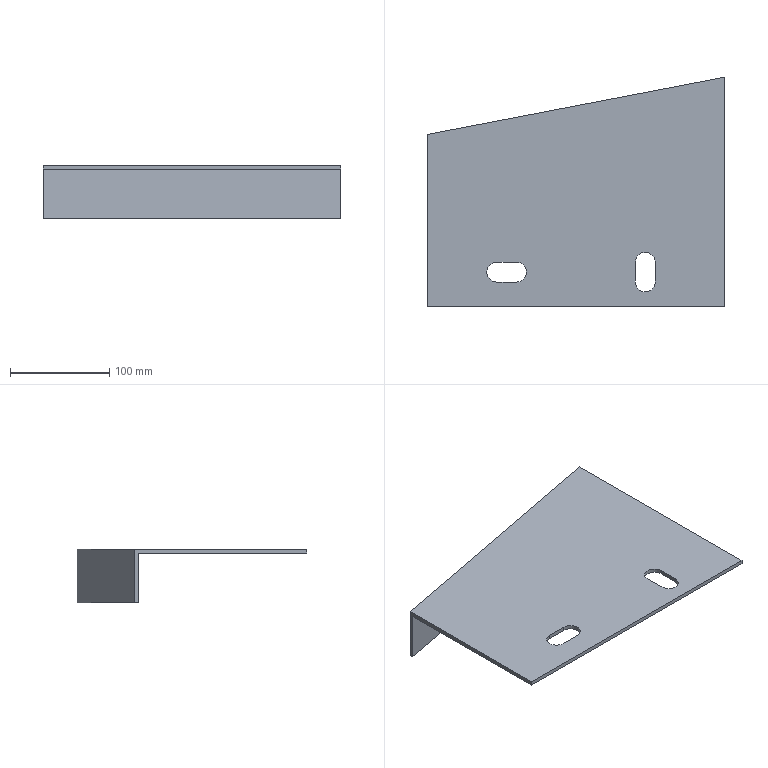Part | SolidWorks | features MirrorStock 1 | 1 solid | 17 faces | box 300 x 231.743 x 54 mm | volume 298834 mm3 | plane 12 | cylinder 5 | commonest cylinder face diameters 20 x5
STEP:
#1=CARTESIAN_POINT('',(60.,35.,-4.));
#2=VERTEX_POINT('',#1);
#3=CARTESIAN_POINT('',(70.,25.,-4.));
#4=VERTEX_POINT('',#3);
#5=CARTESIAN_POINT('',(70.,35.,-4.));
#6=DIRECTION('',(0.,0.,1.));
#7=DIRECTION('',(1.,0.,0.));
#8=AXIS2_PLACEMENT_3D('',#5,#6,#7);
#9=CIRCLE('',#8,10.);
#10=EDGE_CURVE('',#2,#4,#9,.T.);
#11=ORIENTED_EDGE('',*,*,#10,.F.);
#12=CARTESIAN_POINT('',(60.,35.,0.));
#13=VERTEX_POINT('',#12);
#14=CARTESIAN_POINT('',(60.,35.,-4.));
#15=DIRECTION('',(0.,0.,1.));
#16=VECTOR('',#15,1000.);
#17=LINE('',#14,#16);
#18=EDGE_CURVE('',#2,#13,#17,.T.);
#19=ORIENTED_EDGE('',*,*,#18,.T.);
#20=CARTESIAN_POINT('',(70.,25.,0.));
#21=VERTEX_POINT('',#20);
#22=CARTESIAN_POINT('',(70.,35.,0.));
#23=DIRECTION('',(0.,0.,1.));
#24=DIRECTION('',(1.,0.,0.));
#25=AXIS2_PLACEMENT_3D('',#22,#23,#24);
#26=CIRCLE('',#25,10.);
#27=EDGE_CURVE('',#13,#21,#26,.T.);
#28=ORIENTED_EDGE('',*,*,#27,.T.);
#29=CARTESIAN_POINT('',(70.,25.,-4.));
#30=DIRECTION('',(0.,0.,1.));
#31=VECTOR('',#30,1000.);
#32=LINE('',#29,#31);
#33=EDGE_CURVE('',#4,#21,#32,.T.);
#34=ORIENTED_EDGE('',*,*,#33,.F.);
#35=EDGE_LOOP('',(#11,#19,#28,#34));
#36=FACE_OUTER_BOUND('',#35,.T.);
#37=CARTESIAN_POINT('',(70.,35.,-4.));
#38=DIRECTION('',(0.,0.,1.));
#39=DIRECTION('',(-1.,0.,0.));
#40=AXIS2_PLACEMENT_3D('',#37,#38,#39);
#41=CYLINDRICAL_SURFACE('',#40,10.);
#42=ADVANCED_FACE('',(#36),#41,.F.);
#43=CARTESIAN_POINT('',(0.,169.927,-4.));
#44=VERTEX_POINT('',#43);
#45=CARTESIAN_POINT('',(300.,227.669,-4.));
#46=VERTEX_POINT('',#45);
#47=CARTESIAN_POINT('',(21.163,174.,-4.));
#48=DIRECTION('',(0.982,0.189,0.));
#49=VECTOR('',#48,1000.);
#50=LINE('',#47,#49);
#51=EDGE_CURVE('',#44,#46,#50,.T.);
#52=ORIENTED_EDGE('',*,*,#51,.T.);
#53=CARTESIAN_POINT('',(300.,0.,-4.));
#54=VERTEX_POINT('',#53);
#55=CARTESIAN_POINT('',(300.,231.743,-4.));
#56=DIRECTION('',(0.,1.,0.));
#57=VECTOR('',#56,1000.);
#58=LINE('',#55,#57);
#59=EDGE_CURVE('',#54,#46,#58,.T.);
#60=ORIENTED_EDGE('',*,*,#59,.F.);
#61=CARTESIAN_POINT('',(0.,0.,-4.));
#62=VERTEX_POINT('',#61);
#63=CARTESIAN_POINT('',(300.,0.,-4.));
#64=DIRECTION('',(1.,0.,0.));
#65=VECTOR('',#64,1000.);
#66=LINE('',#63,#65);
#67=EDGE_CURVE('',#62,#54,#66,.T.);
#68=ORIENTED_EDGE('',*,*,#67,.F.);
#69=CARTESIAN_POINT('',(0.,0.,-4.));
#70=DIRECTION('',(0.,-1.,0.));
#71=VECTOR('',#70,1000.);
#72=LINE('',#69,#71);
#73=EDGE_CURVE('',#44,#62,#72,.T.);
#74=ORIENTED_EDGE('',*,*,#73,.F.);
#75=EDGE_LOOP('',(#52,#60,#68,#74));
#76=FACE_OUTER_BOUND('',#75,.T.);
#77=CARTESIAN_POINT('',(90.,25.,-4.));
#78=VERTEX_POINT('',#77);
#79=CARTESIAN_POINT('',(90.,25.,-4.));
#80=DIRECTION('',(1.,0.,0.));
#81=VECTOR('',#80,1000.);
#82=LINE('',#79,#81);
#83=EDGE_CURVE('',#4,#78,#82,.T.);
#84=ORIENTED_EDGE('',*,*,#83,.T.);
#85=CARTESIAN_POINT('',(90.,45.,-4.));
#86=VERTEX_POINT('',#85);
#87=CARTESIAN_POINT('',(90.,35.,-4.));
#88=DIRECTION('',(0.,0.,1.));
#89=DIRECTION('',(1.,0.,0.));
#90=AXIS2_PLACEMENT_3D('',#87,#88,#89);
#91=CIRCLE('',#90,10.);
#92=EDGE_CURVE('',#78,#86,#91,.T.);
#93=ORIENTED_EDGE('',*,*,#92,.T.);
#94=CARTESIAN_POINT('',(70.,45.,-4.));
#95=VERTEX_POINT('',#94);
#96=CARTESIAN_POINT('',(70.,45.,-4.));
#97=DIRECTION('',(-1.,0.,0.));
#98=VECTOR('',#97,1000.);
#99=LINE('',#96,#98);
#100=EDGE_CURVE('',#86,#95,#99,.T.);
#101=ORIENTED_EDGE('',*,*,#100,.T.);
#102=CARTESIAN_POINT('',(70.,35.,-4.));
#103=DIRECTION('',(0.,0.,1.));
#104=DIRECTION('',(1.,0.,0.));
#105=AXIS2_PLACEMENT_3D('',#102,#103,#104);
#106=CIRCLE('',#105,10.);
#107=EDGE_CURVE('',#95,#2,#106,.T.);
#108=ORIENTED_EDGE('',*,*,#107,.T.);
#109=ORIENTED_EDGE('',*,*,#10,.T.);
#110=EDGE_LOOP('',(#84,#93,#101,#108,#109));
#111=FACE_BOUND('',#110,.T.);
#112=CARTESIAN_POINT('',(210.,45.,-4.));
#113=VERTEX_POINT('',#112);
#114=CARTESIAN_POINT('',(210.,25.,-4.));
#115=VERTEX_POINT('',#114);
#116=CARTESIAN_POINT('',(210.,25.,-4.));
#117=DIRECTION('',(0.,-1.,0.));
#118=VECTOR('',#117,1000.);
#119=LINE('',#116,#118);
#120=EDGE_CURVE('',#113,#115,#119,.T.);
#121=ORIENTED_EDGE('',*,*,#120,.T.);
#122=CARTESIAN_POINT('',(230.,25.,-4.));
#123=VERTEX_POINT('',#122);
#124=CARTESIAN_POINT('',(220.,25.,-4.));
#125=DIRECTION('',(0.,0.,1.));
#126=DIRECTION('',(1.,0.,0.));
#127=AXIS2_PLACEMENT_3D('',#124,#125,#126);
#128=CIRCLE('',#127,10.);
#129=EDGE_CURVE('',#115,#123,#128,.T.);
#130=ORIENTED_EDGE('',*,*,#129,.T.);
#131=CARTESIAN_POINT('',(230.,45.,-4.));
#132=VERTEX_POINT('',#131);
#133=CARTESIAN_POINT('',(230.,45.,-4.));
#134=DIRECTION('',(0.,1.,0.));
#135=VECTOR('',#134,1000.);
#136=LINE('',#133,#135);
#137=EDGE_CURVE('',#123,#132,#136,.T.);
#138=ORIENTED_EDGE('',*,*,#137,.T.);
#139=CARTESIAN_POINT('',(220.,45.,-4.));
#140=DIRECTION('',(0.,0.,1.));
#141=DIRECTION('',(1.,0.,0.));
#142=AXIS2_PLACEMENT_3D('',#139,#140,#141);
#143=CIRCLE('',#142,10.);
#144=EDGE_CURVE('',#132,#113,#143,.T.);
#145=ORIENTED_EDGE('',*,*,#144,.T.);
#146=EDGE_LOOP('',(#121,#130,#138,#145));
#147=FACE_BOUND('',#146,.T.);
#148=CARTESIAN_POINT('',(0.,0.,-4.));
#149=DIRECTION('',(0.,0.,-1.));
#150=DIRECTION('',(1.,0.,0.));
#151=AXIS2_PLACEMENT_3D('',#148,#149,#150);
#152=PLANE('',#151);
#153=ADVANCED_FACE('',(#76,#111,#147),#152,.T.);
#154=CARTESIAN_POINT('',(70.,45.,0.));
#155=VERTEX_POINT('',#154);
#156=CARTESIAN_POINT('',(70.,35.,0.));
#157=DIRECTION('',(0.,0.,1.));
#158=DIRECTION('',(1.,0.,0.));
#159=AXIS2_PLACEMENT_3D('',#156,#157,#158);
#160=CIRCLE('',#159,10.);
#161=EDGE_CURVE('',#155,#13,#160,.T.);
#162=ORIENTED_EDGE('',*,*,#161,.F.);
#163=CARTESIAN_POINT('',(90.,45.,0.));
#164=VERTEX_POINT('',#163);
#165=CARTESIAN_POINT('',(70.,45.,0.));
#166=DIRECTION('',(-1.,0.,0.));
#167=VECTOR('',#166,1000.);
#168=LINE('',#165,#167);
#169=EDGE_CURVE('',#164,#155,#168,.T.);
#170=ORIENTED_EDGE('',*,*,#169,.F.);
#171=CARTESIAN_POINT('',(90.,25.,0.));
#172=VERTEX_POINT('',#171);
#173=CARTESIAN_POINT('',(90.,35.,0.));
#174=DIRECTION('',(0.,0.,1.));
#175=DIRECTION('',(1.,0.,0.));
#176=AXIS2_PLACEMENT_3D('',#173,#174,#175);
#177=CIRCLE('',#176,10.);
#178=EDGE_CURVE('',#172,#164,#177,.T.);
#179=ORIENTED_EDGE('',*,*,#178,.F.);
#180=CARTESIAN_POINT('',(90.,25.,0.));
#181=DIRECTION('',(1.,0.,0.));
#182=VECTOR('',#181,1000.);
#183=LINE('',#180,#182);
#184=EDGE_CURVE('',#21,#172,#183,.T.);
#185=ORIENTED_EDGE('',*,*,#184,.F.);
#186=ORIENTED_EDGE('',*,*,#27,.F.);
#187=EDGE_LOOP('',(#162,#170,#179,#185,#186));
#188=FACE_BOUND('',#187,.T.);
#189=CARTESIAN_POINT('',(0.,174.,0.));
#190=VERTEX_POINT('',#189);
#191=CARTESIAN_POINT('',(0.,0.,0.));
#192=VERTEX_POINT('',#191);
#193=CARTESIAN_POINT('',(0.,0.,0.));
#194=DIRECTION('',(0.,-1.,0.));
#195=VECTOR('',#194,1000.);
#196=LINE('',#193,#195);
#197=EDGE_CURVE('',#190,#192,#196,.T.);
#198=ORIENTED_EDGE('',*,*,#197,.T.);
#199=CARTESIAN_POINT('',(300.,0.,0.));
#200=VERTEX_POINT('',#199);
#201=CARTESIAN_POINT('',(300.,0.,0.));
#202=DIRECTION('',(1.,0.,0.));
#203=VECTOR('',#202,1000.);
#204=LINE('',#201,#203);
#205=EDGE_CURVE('',#192,#200,#204,.T.);
#206=ORIENTED_EDGE('',*,*,#205,.T.);
#207=CARTESIAN_POINT('',(300.,231.743,0.));
#208=VERTEX_POINT('',#207);
#209=CARTESIAN_POINT('',(300.,231.743,0.));
#210=DIRECTION('',(0.,1.,0.));
#211=VECTOR('',#210,1000.);
#212=LINE('',#209,#211);
#213=EDGE_CURVE('',#200,#208,#212,.T.);
#214=ORIENTED_EDGE('',*,*,#213,.T.);
#215=CARTESIAN_POINT('',(0.,174.,0.));
#216=DIRECTION('',(-0.982,-0.189,0.));
#217=VECTOR('',#216,1000.);
#218=LINE('',#215,#217);
#219=EDGE_CURVE('',#208,#190,#218,.T.);
#220=ORIENTED_EDGE('',*,*,#219,.T.);
#221=EDGE_LOOP('',(#198,#206,#214,#220));
#222=FACE_OUTER_BOUND('',#221,.T.);
#223=CARTESIAN_POINT('',(230.,45.,0.));
#224=VERTEX_POINT('',#223);
#225=CARTESIAN_POINT('',(210.,45.,0.));
#226=VERTEX_POINT('',#225);
#227=CARTESIAN_POINT('',(220.,45.,0.));
#228=DIRECTION('',(0.,0.,1.));
#229=DIRECTION('',(1.,0.,0.));
#230=AXIS2_PLACEMENT_3D('',#227,#228,#229);
#231=CIRCLE('',#230,10.);
#232=EDGE_CURVE('',#224,#226,#231,.T.);
#233=ORIENTED_EDGE('',*,*,#232,.F.);
#234=CARTESIAN_POINT('',(230.,25.,0.));
#235=VERTEX_POINT('',#234);
#236=CARTESIAN_POINT('',(230.,45.,0.));
#237=DIRECTION('',(0.,1.,0.));
#238=VECTOR('',#237,1000.);
#239=LINE('',#236,#238);
#240=EDGE_CURVE('',#235,#224,#239,.T.);
#241=ORIENTED_EDGE('',*,*,#240,.F.);
#242=CARTESIAN_POINT('',(210.,25.,0.));
#243=VERTEX_POINT('',#242);
#244=CARTESIAN_POINT('',(220.,25.,0.));
#245=DIRECTION('',(0.,0.,1.));
#246=DIRECTION('',(1.,0.,0.));
#247=AXIS2_PLACEMENT_3D('',#244,#245,#246);
#248=CIRCLE('',#247,10.);
#249=EDGE_CURVE('',#243,#235,#248,.T.);
#250=ORIENTED_EDGE('',*,*,#249,.F.);
#251=CARTESIAN_POINT('',(210.,25.,0.));
#252=DIRECTION('',(0.,-1.,0.));
#253=VECTOR('',#252,1000.);
#254=LINE('',#251,#253);
#255=EDGE_CURVE('',#226,#243,#254,.T.);
#256=ORIENTED_EDGE('',*,*,#255,.F.);
#257=EDGE_LOOP('',(#233,#241,#250,#256));
#258=FACE_BOUND('',#257,.T.);
#259=CARTESIAN_POINT('',(0.,0.,0.));
#260=DIRECTION('',(0.,0.,-1.));
#261=DIRECTION('',(1.,0.,0.));
#262=AXIS2_PLACEMENT_3D('',#259,#260,#261);
#263=PLANE('',#262);
#264=ADVANCED_FACE('',(#188,#222,#258),#263,.F.);
#265=ORIENTED_EDGE('',*,*,#197,.F.);
#266=CARTESIAN_POINT('',(0.,174.,-54.));
#267=VERTEX_POINT('',#266);
#268=CARTESIAN_POINT('',(0.,174.,-4.));
#269=DIRECTION('',(0.,0.,1.));
#270=VECTOR('',#269,1000.);
#271=LINE('',#268,#270);
#272=EDGE_CURVE('',#267,#190,#271,.T.);
#273=ORIENTED_EDGE('',*,*,#272,.F.);
#274=CARTESIAN_POINT('',(0.,169.927,-54.));
#275=VERTEX_POINT('',#274);
#276=CARTESIAN_POINT('',(0.,174.,-54.));
#277=DIRECTION('',(0.,-1.,0.));
#278=VECTOR('',#277,1000.);
#279=LINE('',#276,#278);
#280=EDGE_CURVE('',#267,#275,#279,.T.);
#281=ORIENTED_EDGE('',*,*,#280,.T.);
#282=CARTESIAN_POINT('',(0.,169.927,-54.));
#283=DIRECTION('',(0.,0.,1.));
#284=VECTOR('',#283,1000.);
#285=LINE('',#282,#284);
#286=EDGE_CURVE('',#275,#44,#285,.T.);
#287=ORIENTED_EDGE('',*,*,#286,.T.);
#288=ORIENTED_EDGE('',*,*,#73,.T.);
#289=CARTESIAN_POINT('',(0.,0.,-4.));
#290=DIRECTION('',(0.,0.,1.));
#291=VECTOR('',#290,1000.);
#292=LINE('',#289,#291);
#293=EDGE_CURVE('',#62,#192,#292,.T.);
#294=ORIENTED_EDGE('',*,*,#293,.T.);
#295=EDGE_LOOP('',(#265,#273,#281,#287,#288,#294));
#296=FACE_OUTER_BOUND('',#295,.T.);
#297=CARTESIAN_POINT('',(0.,0.,-4.));
#298=DIRECTION('',(1.,0.,0.));
#299=DIRECTION('',(0.,1.,0.));
#300=AXIS2_PLACEMENT_3D('',#297,#298,#299);
#301=PLANE('',#300);
#302=ADVANCED_FACE('',(#296),#301,.F.);
#303=ORIENTED_EDGE('',*,*,#205,.F.);
#304=ORIENTED_EDGE('',*,*,#293,.F.);
#305=ORIENTED_EDGE('',*,*,#67,.T.);
#306=CARTESIAN_POINT('',(300.,0.,-4.));
#307=DIRECTION('',(0.,0.,1.));
#308=VECTOR('',#307,1000.);
#309=LINE('',#306,#308);
#310=EDGE_CURVE('',#54,#200,#309,.T.);
#311=ORIENTED_EDGE('',*,*,#310,.T.);
#312=EDGE_LOOP('',(#303,#304,#305,#311));
#313=FACE_OUTER_BOUND('',#312,.T.);
#314=CARTESIAN_POINT('',(300.,0.,-4.));
#315=DIRECTION('',(0.,1.,0.));
#316=DIRECTION('',(0.,0.,-1.));
#317=AXIS2_PLACEMENT_3D('',#314,#315,#316);
#318=PLANE('',#317);
#319=ADVANCED_FACE('',(#313),#318,.F.);
#320=ORIENTED_EDGE('',*,*,#213,.F.);
#321=ORIENTED_EDGE('',*,*,#310,.F.);
#322=ORIENTED_EDGE('',*,*,#59,.T.);
#323=CARTESIAN_POINT('',(300.,227.669,-54.));
#324=VERTEX_POINT('',#323);
#325=CARTESIAN_POINT('',(300.,227.669,-54.));
#326=DIRECTION('',(0.,0.,1.));
#327=VECTOR('',#326,1000.);
#328=LINE('',#325,#327);
#329=EDGE_CURVE('',#324,#46,#328,.T.);
#330=ORIENTED_EDGE('',*,*,#329,.F.);
#331=CARTESIAN_POINT('',(300.,231.743,-54.));
#332=VERTEX_POINT('',#331);
#333=CARTESIAN_POINT('',(300.,227.669,-54.));
#334=DIRECTION('',(0.,1.,0.));
#335=VECTOR('',#334,1000.);
#336=LINE('',#333,#335);
#337=EDGE_CURVE('',#324,#332,#336,.T.);
#338=ORIENTED_EDGE('',*,*,#337,.T.);
#339=CARTESIAN_POINT('',(300.,231.743,-4.));
#340=DIRECTION('',(0.,0.,1.));
#341=VECTOR('',#340,1000.);
#342=LINE('',#339,#341);
#343=EDGE_CURVE('',#332,#208,#342,.T.);
#344=ORIENTED_EDGE('',*,*,#343,.T.);
#345=EDGE_LOOP('',(#320,#321,#322,#330,#338,#344));
#346=FACE_OUTER_BOUND('',#345,.T.);
#347=CARTESIAN_POINT('',(300.,231.743,-4.));
#348=DIRECTION('',(-1.,0.,0.));
#349=DIRECTION('',(0.,0.,-1.));
#350=AXIS2_PLACEMENT_3D('',#347,#348,#349);
#351=PLANE('',#350);
#352=ADVANCED_FACE('',(#346),#351,.F.);
#353=ORIENTED_EDGE('',*,*,#219,.F.);
#354=ORIENTED_EDGE('',*,*,#343,.F.);
#355=CARTESIAN_POINT('',(300.,231.743,-54.));
#356=DIRECTION('',(-0.982,-0.189,0.));
#357=VECTOR('',#356,1000.);
#358=LINE('',#355,#357);
#359=EDGE_CURVE('',#332,#267,#358,.T.);
#360=ORIENTED_EDGE('',*,*,#359,.T.);
#361=ORIENTED_EDGE('',*,*,#272,.T.);
#362=EDGE_LOOP('',(#353,#354,#360,#361));
#363=FACE_OUTER_BOUND('',#362,.T.);
#364=CARTESIAN_POINT('',(0.,174.,-4.));
#365=DIRECTION('',(0.189,-0.982,0.));
#366=DIRECTION('',(0.982,0.189,0.));
#367=AXIS2_PLACEMENT_3D('',#364,#365,#366);
#368=PLANE('',#367);
#369=ADVANCED_FACE('',(#363),#368,.F.);
#370=ORIENTED_EDGE('',*,*,#18,.F.);
#371=ORIENTED_EDGE('',*,*,#107,.F.);
#372=CARTESIAN_POINT('',(70.,45.,-4.));
#373=DIRECTION('',(0.,0.,1.));
#374=VECTOR('',#373,1000.);
#375=LINE('',#372,#374);
#376=EDGE_CURVE('',#95,#155,#375,.T.);
#377=ORIENTED_EDGE('',*,*,#376,.T.);
#378=ORIENTED_EDGE('',*,*,#161,.T.);
#379=EDGE_LOOP('',(#370,#371,#377,#378));
#380=FACE_OUTER_BOUND('',#379,.T.);
#381=CARTESIAN_POINT('',(70.,35.,-4.));
#382=DIRECTION('',(0.,0.,1.));
#383=DIRECTION('',(-1.,0.,0.));
#384=AXIS2_PLACEMENT_3D('',#381,#382,#383);
#385=CYLINDRICAL_SURFACE('',#384,10.);
#386=ADVANCED_FACE('',(#380),#385,.F.);
#387=ORIENTED_EDGE('',*,*,#184,.T.);
#388=CARTESIAN_POINT('',(90.,25.,-4.));
#389=DIRECTION('',(0.,0.,1.));
#390=VECTOR('',#389,1000.);
#391=LINE('',#388,#390);
#392=EDGE_CURVE('',#78,#172,#391,.T.);
#393=ORIENTED_EDGE('',*,*,#392,.F.);
#394=ORIENTED_EDGE('',*,*,#83,.F.);
#395=ORIENTED_EDGE('',*,*,#33,.T.);
#396=EDGE_LOOP('',(#387,#393,#394,#395));
#397=FACE_OUTER_BOUND('',#396,.T.);
#398=CARTESIAN_POINT('',(90.,25.,-4.));
#399=DIRECTION('',(0.,1.,0.));
#400=DIRECTION('',(0.,0.,-1.));
#401=AXIS2_PLACEMENT_3D('',#398,#399,#400);
#402=PLANE('',#401);
#403=ADVANCED_FACE('',(#397),#402,.T.);
#404=ORIENTED_EDGE('',*,*,#178,.T.);
#405=CARTESIAN_POINT('',(90.,45.,-4.));
#406=DIRECTION('',(0.,0.,1.));
#407=VECTOR('',#406,1000.);
#408=LINE('',#405,#407);
#409=EDGE_CURVE('',#86,#164,#408,.T.);
#410=ORIENTED_EDGE('',*,*,#409,.F.);
#411=ORIENTED_EDGE('',*,*,#92,.F.);
#412=ORIENTED_EDGE('',*,*,#392,.T.);
#413=EDGE_LOOP('',(#404,#410,#411,#412));
#414=FACE_OUTER_BOUND('',#413,.T.);
#415=CARTESIAN_POINT('',(90.,35.,-4.));
#416=DIRECTION('',(0.,0.,1.));
#417=DIRECTION('',(-1.,0.,0.));
#418=AXIS2_PLACEMENT_3D('',#415,#416,#417);
#419=CYLINDRICAL_SURFACE('',#418,10.);
#420=ADVANCED_FACE('',(#414),#419,.F.);
#421=ORIENTED_EDGE('',*,*,#169,.T.);
#422=ORIENTED_EDGE('',*,*,#376,.F.);
#423=ORIENTED_EDGE('',*,*,#100,.F.);
#424=ORIENTED_EDGE('',*,*,#409,.T.);
#425=EDGE_LOOP('',(#421,#422,#423,#424));
#426=FACE_OUTER_BOUND('',#425,.T.);
#427=CARTESIAN_POINT('',(70.,45.,-4.));
#428=DIRECTION('',(0.,-1.,0.));
#429=DIRECTION('',(0.,0.,1.));
#430=AXIS2_PLACEMENT_3D('',#427,#428,#429);
#431=PLANE('',#430);
#432=ADVANCED_FACE('',(#426),#431,.T.);
#433=ORIENTED_EDGE('',*,*,#232,.T.);
#434=CARTESIAN_POINT('',(210.,45.,-4.));
#435=DIRECTION('',(0.,0.,1.));
#436=VECTOR('',#435,1000.);
#437=LINE('',#434,#436);
#438=EDGE_CURVE('',#113,#226,#437,.T.);
#439=ORIENTED_EDGE('',*,*,#438,.F.);
#440=ORIENTED_EDGE('',*,*,#144,.F.);
#441=CARTESIAN_POINT('',(230.,45.,-4.));
#442=DIRECTION('',(0.,0.,1.));
#443=VECTOR('',#442,1000.);
#444=LINE('',#441,#443);
#445=EDGE_CURVE('',#132,#224,#444,.T.);
#446=ORIENTED_EDGE('',*,*,#445,.T.);
#447=EDGE_LOOP('',(#433,#439,#440,#446));
#448=FACE_OUTER_BOUND('',#447,.T.);
#449=CARTESIAN_POINT('',(220.,45.,-4.));
#450=DIRECTION('',(0.,0.,1.));
#451=DIRECTION('',(-1.,0.,0.));
#452=AXIS2_PLACEMENT_3D('',#449,#450,#451);
#453=CYLINDRICAL_SURFACE('',#452,10.);
#454=ADVANCED_FACE('',(#448),#453,.F.);
#455=ORIENTED_EDGE('',*,*,#255,.T.);
#456=CARTESIAN_POINT('',(210.,25.,-4.));
#457=DIRECTION('',(0.,0.,1.));
#458=VECTOR('',#457,1000.);
#459=LINE('',#456,#458);
#460=EDGE_CURVE('',#115,#243,#459,.T.);
#461=ORIENTED_EDGE('',*,*,#460,.F.);
#462=ORIENTED_EDGE('',*,*,#120,.F.);
#463=ORIENTED_EDGE('',*,*,#438,.T.);
#464=EDGE_LOOP('',(#455,#461,#462,#463));
#465=FACE_OUTER_BOUND('',#464,.T.);
#466=CARTESIAN_POINT('',(210.,25.,-4.));
#467=DIRECTION('',(1.,0.,0.));
#468=DIRECTION('',(0.,0.,1.));
#469=AXIS2_PLACEMENT_3D('',#466,#467,#468);
#470=PLANE('',#469);
#471=ADVANCED_FACE('',(#465),#470,.T.);
#472=ORIENTED_EDGE('',*,*,#249,.T.);
#473=CARTESIAN_POINT('',(230.,25.,-4.));
#474=DIRECTION('',(0.,0.,1.));
#475=VECTOR('',#474,1000.);
#476=LINE('',#473,#475);
#477=EDGE_CURVE('',#123,#235,#476,.T.);
#478=ORIENTED_EDGE('',*,*,#477,.F.);
#479=ORIENTED_EDGE('',*,*,#129,.F.);
#480=ORIENTED_EDGE('',*,*,#460,.T.);
#481=EDGE_LOOP('',(#472,#478,#479,#480));
#482=FACE_OUTER_BOUND('',#481,.T.);
#483=CARTESIAN_POINT('',(220.,25.,-4.));
#484=DIRECTION('',(0.,0.,1.));
#485=DIRECTION('',(-1.,0.,0.));
#486=AXIS2_PLACEMENT_3D('',#483,#484,#485);
#487=CYLINDRICAL_SURFACE('',#486,10.);
#488=ADVANCED_FACE('',(#482),#487,.F.);
#489=ORIENTED_EDGE('',*,*,#240,.T.);
#490=ORIENTED_EDGE('',*,*,#445,.F.);
#491=ORIENTED_EDGE('',*,*,#137,.F.);
#492=ORIENTED_EDGE('',*,*,#477,.T.);
#493=EDGE_LOOP('',(#489,#490,#491,#492));
#494=FACE_OUTER_BOUND('',#493,.T.);
#495=CARTESIAN_POINT('',(230.,45.,-4.));
#496=DIRECTION('',(-1.,0.,0.));
#497=DIRECTION('',(0.,0.,-1.));
#498=AXIS2_PLACEMENT_3D('',#495,#496,#497);
#499=PLANE('',#498);
#500=ADVANCED_FACE('',(#494),#499,.T.);
#501=ORIENTED_EDGE('',*,*,#51,.F.);
#502=ORIENTED_EDGE('',*,*,#286,.F.);
#503=CARTESIAN_POINT('',(0.,169.927,-54.));
#504=DIRECTION('',(0.982,0.189,0.));
#505=VECTOR('',#504,1000.);
#506=LINE('',#503,#505);
#507=EDGE_CURVE('',#275,#324,#506,.T.);
#508=ORIENTED_EDGE('',*,*,#507,.T.);
#509=ORIENTED_EDGE('',*,*,#329,.T.);
#510=EDGE_LOOP('',(#501,#502,#508,#509));
#511=FACE_OUTER_BOUND('',#510,.T.);
#512=CARTESIAN_POINT('',(21.163,174.,-54.));
#513=DIRECTION('',(-0.189,0.982,0.));
#514=DIRECTION('',(-0.982,-0.189,0.));
#515=AXIS2_PLACEMENT_3D('',#512,#513,#514);
#516=PLANE('',#515);
#517=ADVANCED_FACE('',(#511),#516,.F.);
#518=ORIENTED_EDGE('',*,*,#280,.F.);
#519=ORIENTED_EDGE('',*,*,#359,.F.);
#520=ORIENTED_EDGE('',*,*,#337,.F.);
#521=ORIENTED_EDGE('',*,*,#507,.F.);
#522=EDGE_LOOP('',(#518,#519,#520,#521));
#523=FACE_OUTER_BOUND('',#522,.T.);
#524=CARTESIAN_POINT('',(0.,0.,-54.));
#525=DIRECTION('',(0.,0.,-1.));
#526=DIRECTION('',(1.,0.,0.));
#527=AXIS2_PLACEMENT_3D('',#524,#525,#526);
#528=PLANE('',#527);
#529=ADVANCED_FACE('',(#523),#528,.T.);
#530=CLOSED_SHELL('',(#42,#153,#264,#302,#319,#352,#369,#386,#403,#420,#432,#454,#471,#488,#500,#517,#529));
#531=MANIFOLD_SOLID_BREP('',#530);
#532=CARTESIAN_POINT('',(0.,0.,0.));
#533=DIRECTION('',(0.,0.,1.));
#534=DIRECTION('',(1.,0.,0.));
#535=AXIS2_PLACEMENT_3D('',#532,#533,#534);
#536=(LENGTH_UNIT()NAMED_UNIT(*)SI_UNIT(.MILLI.,.METRE.));
#537=UNCERTAINTY_MEASURE_WITH_UNIT(LENGTH_MEASURE(0.00001),#536,'','');
#538=(NAMED_UNIT(*)PLANE_ANGLE_UNIT()SI_UNIT($,.RADIAN.));
#539=(NAMED_UNIT(*)SI_UNIT($,.STERADIAN.)SOLID_ANGLE_UNIT());
#540=(GEOMETRIC_REPRESENTATION_CONTEXT(3)GLOBAL_UNCERTAINTY_ASSIGNED_CONTEXT((#537))GLOBAL_UNIT_ASSIGNED_CONTEXT((#536,#538,#539))REPRESENTATION_CONTEXT('',''));
#541=ADVANCED_BREP_SHAPE_REPRESENTATION('',(#531,#535),#540);